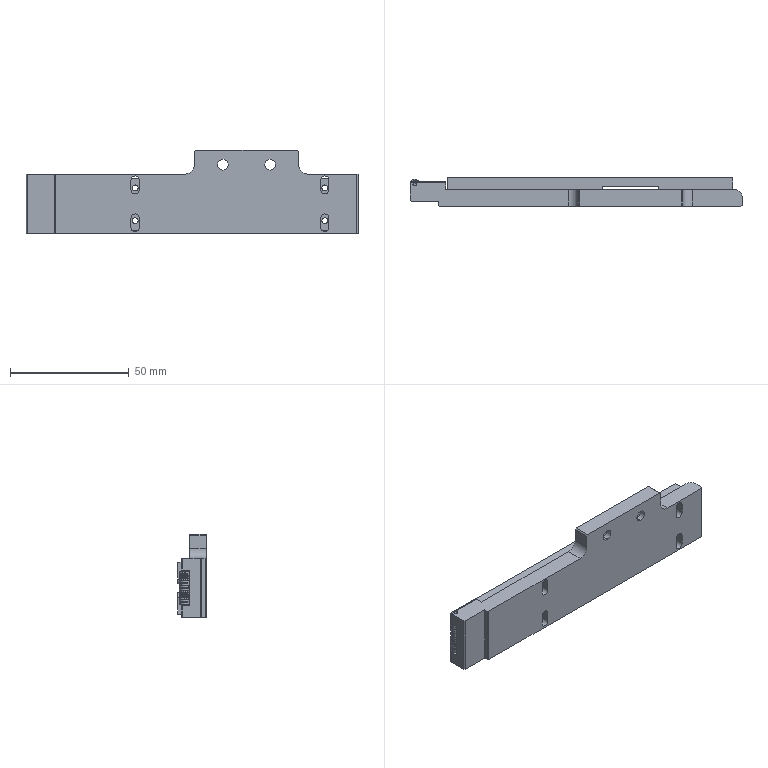Part | SolidWorks | features AEMSimFeature 1, CompositeCurve 1 | 12 solids | 1064 faces | box 140 x 12 x 35 mm | volume 35220 mm3 | plane 413 | torus 308 | sphere 168 | cylinder 135 | spline 32 | cone 8 | commonest cylinder face diameters 2.333 x28 3.167 x28 4 x22 1.5 x18 2.5 x12 3.5 x12